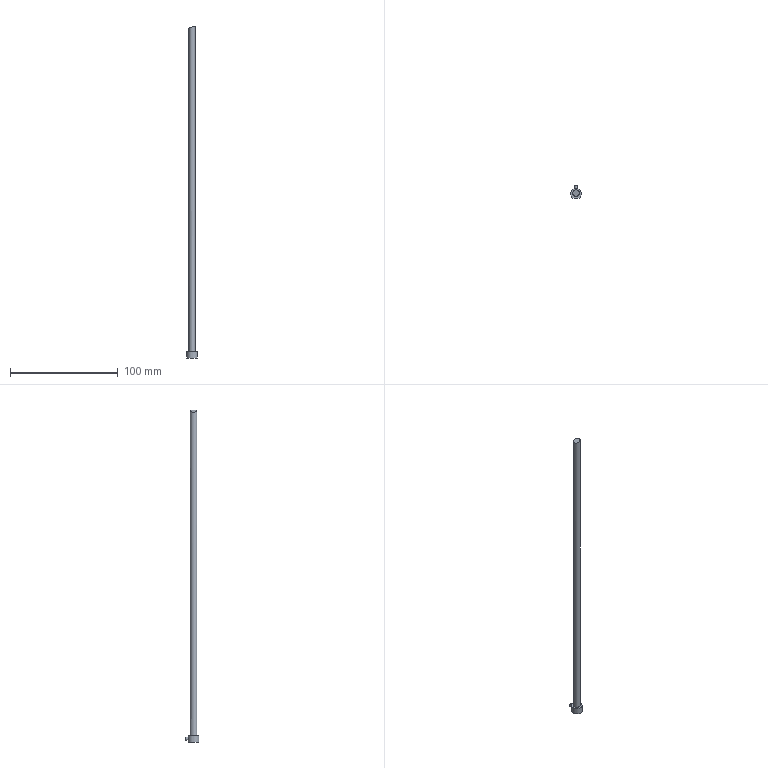Part | STEP file | E106-23-315 | 1 solid | 8 faces | box 10 x 13 x 307.684 mm | volume 8994 mm3 | cylinder 3 | plane 3 | spline 1 | cone 1 | commonest cylinder face diameters 3 x1 6 x1 10 x1